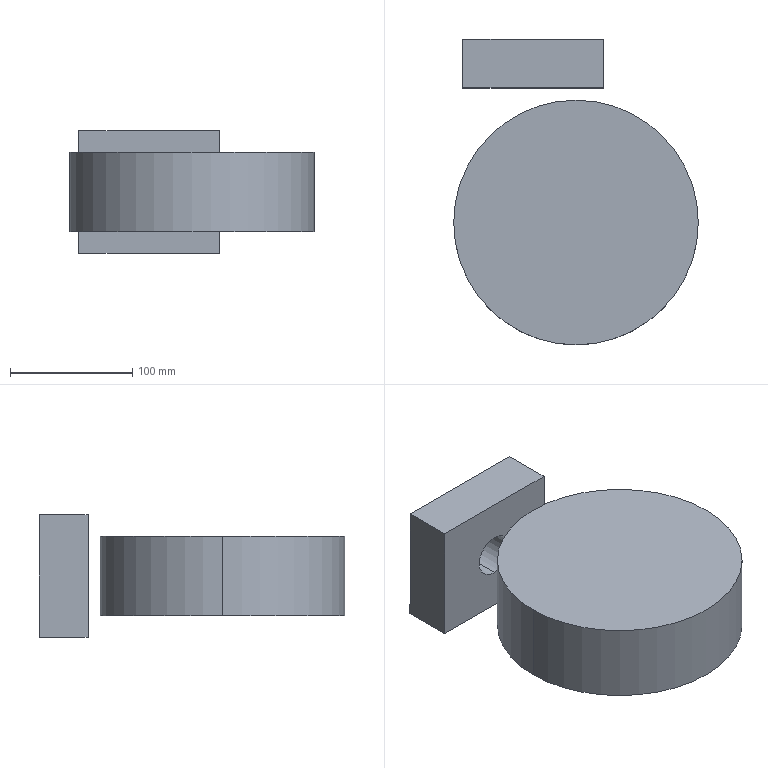Part | SolidWorks | features ICE 2, Extrusion 1 | 2 solids | 12 faces | box 200 x 250 x 100 mm | volume 2463636 mm3 | plane 8 | cylinder 4 | commonest cylinder face diameters 34.961 x2 200 x2
STEP:
#1=CARTESIAN_POINT('',(100.,0.,32.5));
#2=VERTEX_POINT('',#1);
#3=CARTESIAN_POINT('',(-100.,0.,32.5));
#4=VERTEX_POINT('',#3);
#5=CARTESIAN_POINT('',(0.,0.,32.5));
#6=DIRECTION('',(0.,0.,1.));
#7=DIRECTION('',(1.,0.,0.));
#8=AXIS2_PLACEMENT_3D('',#5,#6,#7);
#9=CIRCLE('',#8,100.);
#10=EDGE_CURVE('',#2,#4,#9,.T.);
#11=ORIENTED_EDGE('',*,*,#10,.F.);
#12=CARTESIAN_POINT('',(100.,0.,-32.5));
#13=VERTEX_POINT('',#12);
#14=CARTESIAN_POINT('',(100.,0.,32.5));
#15=DIRECTION('',(0.,0.,-1.));
#16=VECTOR('',#15,1000.);
#17=LINE('',#14,#16);
#18=EDGE_CURVE('',#2,#13,#17,.T.);
#19=ORIENTED_EDGE('',*,*,#18,.T.);
#20=CARTESIAN_POINT('',(-100.,0.,-32.5));
#21=VERTEX_POINT('',#20);
#22=CARTESIAN_POINT('',(0.,0.,-32.5));
#23=DIRECTION('',(0.,0.,1.));
#24=DIRECTION('',(1.,0.,0.));
#25=AXIS2_PLACEMENT_3D('',#22,#23,#24);
#26=CIRCLE('',#25,100.);
#27=EDGE_CURVE('',#13,#21,#26,.T.);
#28=ORIENTED_EDGE('',*,*,#27,.T.);
#29=CARTESIAN_POINT('',(-100.,0.,32.5));
#30=DIRECTION('',(0.,0.,-1.));
#31=VECTOR('',#30,1000.);
#32=LINE('',#29,#31);
#33=EDGE_CURVE('',#4,#21,#32,.T.);
#34=ORIENTED_EDGE('',*,*,#33,.F.);
#35=EDGE_LOOP('',(#11,#19,#28,#34));
#36=FACE_OUTER_BOUND('',#35,.T.);
#37=CARTESIAN_POINT('',(0.,0.,32.5));
#38=DIRECTION('',(0.,0.,-1.));
#39=DIRECTION('',(-1.,0.,0.));
#40=AXIS2_PLACEMENT_3D('',#37,#38,#39);
#41=CYLINDRICAL_SURFACE('',#40,100.);
#42=ADVANCED_FACE('',(#36),#41,.T.);
#43=ORIENTED_EDGE('',*,*,#18,.F.);
#44=CARTESIAN_POINT('',(0.,0.,32.5));
#45=DIRECTION('',(0.,0.,1.));
#46=DIRECTION('',(1.,0.,0.));
#47=AXIS2_PLACEMENT_3D('',#44,#45,#46);
#48=CIRCLE('',#47,100.);
#49=EDGE_CURVE('',#4,#2,#48,.T.);
#50=ORIENTED_EDGE('',*,*,#49,.F.);
#51=ORIENTED_EDGE('',*,*,#33,.T.);
#52=CARTESIAN_POINT('',(0.,0.,-32.5));
#53=DIRECTION('',(0.,0.,1.));
#54=DIRECTION('',(1.,0.,0.));
#55=AXIS2_PLACEMENT_3D('',#52,#53,#54);
#56=CIRCLE('',#55,100.);
#57=EDGE_CURVE('',#21,#13,#56,.T.);
#58=ORIENTED_EDGE('',*,*,#57,.T.);
#59=EDGE_LOOP('',(#43,#50,#51,#58));
#60=FACE_OUTER_BOUND('',#59,.T.);
#61=CARTESIAN_POINT('',(0.,0.,32.5));
#62=DIRECTION('',(0.,0.,-1.));
#63=DIRECTION('',(-1.,0.,0.));
#64=AXIS2_PLACEMENT_3D('',#61,#62,#63);
#65=CYLINDRICAL_SURFACE('',#64,100.);
#66=ADVANCED_FACE('',(#60),#65,.T.);
#67=ORIENTED_EDGE('',*,*,#49,.T.);
#68=ORIENTED_EDGE('',*,*,#10,.T.);
#69=EDGE_LOOP('',(#67,#68));
#70=FACE_OUTER_BOUND('',#69,.T.);
#71=CARTESIAN_POINT('',(0.,0.,32.5));
#72=DIRECTION('',(0.,0.,1.));
#73=DIRECTION('',(1.,0.,0.));
#74=AXIS2_PLACEMENT_3D('',#71,#72,#73);
#75=PLANE('',#74);
#76=ADVANCED_FACE('',(#70),#75,.T.);
#77=ORIENTED_EDGE('',*,*,#57,.F.);
#78=ORIENTED_EDGE('',*,*,#27,.F.);
#79=EDGE_LOOP('',(#77,#78));
#80=FACE_OUTER_BOUND('',#79,.T.);
#81=CARTESIAN_POINT('',(0.,0.,-32.5));
#82=DIRECTION('',(0.,0.,1.));
#83=DIRECTION('',(1.,0.,0.));
#84=AXIS2_PLACEMENT_3D('',#81,#82,#83);
#85=PLANE('',#84);
#86=ADVANCED_FACE('',(#80),#85,.F.);
#87=CLOSED_SHELL('',(#42,#66,#76,#86));
#88=MANIFOLD_SOLID_BREP('',#87);
#89=CARTESIAN_POINT('',(-35.,110.,17.481));
#90=VERTEX_POINT('',#89);
#91=CARTESIAN_POINT('',(-35.,110.,-17.481));
#92=VERTEX_POINT('',#91);
#93=CARTESIAN_POINT('',(-35.,110.,0.));
#94=DIRECTION('',(0.,-1.,0.));
#95=DIRECTION('',(-1.,0.,0.));
#96=AXIS2_PLACEMENT_3D('',#93,#94,#95);
#97=CIRCLE('',#96,17.481);
#98=EDGE_CURVE('',#90,#92,#97,.T.);
#99=ORIENTED_EDGE('',*,*,#98,.T.);
#100=CARTESIAN_POINT('',(-35.,150.,-17.481));
#101=VERTEX_POINT('',#100);
#102=CARTESIAN_POINT('',(-35.,-100.001,-17.481));
#103=DIRECTION('',(0.,1.,0.));
#104=VECTOR('',#103,1000.);
#105=LINE('',#102,#104);
#106=EDGE_CURVE('',#92,#101,#105,.T.);
#107=ORIENTED_EDGE('',*,*,#106,.T.);
#108=CARTESIAN_POINT('',(-35.,150.,17.481));
#109=VERTEX_POINT('',#108);
#110=CARTESIAN_POINT('',(-35.,150.,0.));
#111=DIRECTION('',(0.,1.,0.));
#112=DIRECTION('',(0.,0.,1.));
#113=AXIS2_PLACEMENT_3D('',#110,#111,#112);
#114=CIRCLE('',#113,17.481);
#115=EDGE_CURVE('',#101,#109,#114,.T.);
#116=ORIENTED_EDGE('',*,*,#115,.T.);
#117=CARTESIAN_POINT('',(-35.,-100.001,17.481));
#118=DIRECTION('',(0.,1.,0.));
#119=VECTOR('',#118,1000.);
#120=LINE('',#117,#119);
#121=EDGE_CURVE('',#90,#109,#120,.T.);
#122=ORIENTED_EDGE('',*,*,#121,.F.);
#123=EDGE_LOOP('',(#99,#107,#116,#122));
#124=FACE_OUTER_BOUND('',#123,.T.);
#125=CARTESIAN_POINT('',(-35.,-100.001,0.));
#126=DIRECTION('',(0.,1.,0.));
#127=DIRECTION('',(0.,0.,1.));
#128=AXIS2_PLACEMENT_3D('',#125,#126,#127);
#129=CYLINDRICAL_SURFACE('',#128,17.481);
#130=ADVANCED_FACE('',(#124),#129,.F.);
#131=CARTESIAN_POINT('',(-92.5,150.,-50.));
#132=VERTEX_POINT('',#131);
#133=CARTESIAN_POINT('',(-92.5,110.,-50.));
#134=VERTEX_POINT('',#133);
#135=CARTESIAN_POINT('',(-92.5,150.,-50.));
#136=DIRECTION('',(0.,-1.,0.));
#137=VECTOR('',#136,1000.);
#138=LINE('',#135,#137);
#139=EDGE_CURVE('',#132,#134,#138,.T.);
#140=ORIENTED_EDGE('',*,*,#139,.T.);
#141=CARTESIAN_POINT('',(-92.5,110.,50.));
#142=VERTEX_POINT('',#141);
#143=CARTESIAN_POINT('',(-92.5,110.,50.));
#144=DIRECTION('',(0.,0.,-1.));
#145=VECTOR('',#144,1000.);
#146=LINE('',#143,#145);
#147=EDGE_CURVE('',#142,#134,#146,.T.);
#148=ORIENTED_EDGE('',*,*,#147,.F.);
#149=CARTESIAN_POINT('',(-92.5,150.,50.));
#150=VERTEX_POINT('',#149);
#151=CARTESIAN_POINT('',(-92.5,150.,50.));
#152=DIRECTION('',(0.,-1.,0.));
#153=VECTOR('',#152,1000.);
#154=LINE('',#151,#153);
#155=EDGE_CURVE('',#150,#142,#154,.T.);
#156=ORIENTED_EDGE('',*,*,#155,.F.);
#157=CARTESIAN_POINT('',(-92.5,150.,50.));
#158=DIRECTION('',(0.,0.,-1.));
#159=VECTOR('',#158,1000.);
#160=LINE('',#157,#159);
#161=EDGE_CURVE('',#150,#132,#160,.T.);
#162=ORIENTED_EDGE('',*,*,#161,.T.);
#163=EDGE_LOOP('',(#140,#148,#156,#162));
#164=FACE_OUTER_BOUND('',#163,.T.);
#165=CARTESIAN_POINT('',(-92.5,150.,50.));
#166=DIRECTION('',(1.,0.,0.));
#167=DIRECTION('',(0.,1.,0.));
#168=AXIS2_PLACEMENT_3D('',#165,#166,#167);
#169=PLANE('',#168);
#170=ADVANCED_FACE('',(#164),#169,.F.);
#171=ORIENTED_EDGE('',*,*,#98,.F.);
#172=CARTESIAN_POINT('',(-35.,110.,0.));
#173=DIRECTION('',(0.,-1.,0.));
#174=DIRECTION('',(-1.,0.,0.));
#175=AXIS2_PLACEMENT_3D('',#172,#173,#174);
#176=CIRCLE('',#175,17.481);
#177=EDGE_CURVE('',#92,#90,#176,.T.);
#178=ORIENTED_EDGE('',*,*,#177,.F.);
#179=EDGE_LOOP('',(#171,#178));
#180=FACE_BOUND('',#179,.T.);
#181=CARTESIAN_POINT('',(22.5,110.,-50.));
#182=VERTEX_POINT('',#181);
#183=CARTESIAN_POINT('',(-92.5,110.,-50.));
#184=DIRECTION('',(1.,0.,0.));
#185=VECTOR('',#184,1000.);
#186=LINE('',#183,#185);
#187=EDGE_CURVE('',#134,#182,#186,.T.);
#188=ORIENTED_EDGE('',*,*,#187,.T.);
#189=CARTESIAN_POINT('',(22.5,110.,50.));
#190=VERTEX_POINT('',#189);
#191=CARTESIAN_POINT('',(22.5,110.,50.));
#192=DIRECTION('',(0.,0.,-1.));
#193=VECTOR('',#192,1000.);
#194=LINE('',#191,#193);
#195=EDGE_CURVE('',#190,#182,#194,.T.);
#196=ORIENTED_EDGE('',*,*,#195,.F.);
#197=CARTESIAN_POINT('',(-92.5,110.,50.));
#198=DIRECTION('',(1.,0.,0.));
#199=VECTOR('',#198,1000.);
#200=LINE('',#197,#199);
#201=EDGE_CURVE('',#142,#190,#200,.T.);
#202=ORIENTED_EDGE('',*,*,#201,.F.);
#203=ORIENTED_EDGE('',*,*,#147,.T.);
#204=EDGE_LOOP('',(#188,#196,#202,#203));
#205=FACE_OUTER_BOUND('',#204,.T.);
#206=CARTESIAN_POINT('',(-92.5,110.,50.));
#207=DIRECTION('',(0.,1.,0.));
#208=DIRECTION('',(-1.,0.,0.));
#209=AXIS2_PLACEMENT_3D('',#206,#207,#208);
#210=PLANE('',#209);
#211=ADVANCED_FACE('',(#180,#205),#210,.F.);
#212=CARTESIAN_POINT('',(22.5,150.,-50.));
#213=VERTEX_POINT('',#212);
#214=CARTESIAN_POINT('',(22.5,150.,-50.));
#215=DIRECTION('',(0.,1.,0.));
#216=VECTOR('',#215,1000.);
#217=LINE('',#214,#216);
#218=EDGE_CURVE('',#182,#213,#217,.T.);
#219=ORIENTED_EDGE('',*,*,#218,.T.);
#220=CARTESIAN_POINT('',(22.5,150.,50.));
#221=VERTEX_POINT('',#220);
#222=CARTESIAN_POINT('',(22.5,150.,50.));
#223=DIRECTION('',(0.,0.,-1.));
#224=VECTOR('',#223,1000.);
#225=LINE('',#222,#224);
#226=EDGE_CURVE('',#221,#213,#225,.T.);
#227=ORIENTED_EDGE('',*,*,#226,.F.);
#228=CARTESIAN_POINT('',(22.5,150.,50.));
#229=DIRECTION('',(0.,1.,0.));
#230=VECTOR('',#229,1000.);
#231=LINE('',#228,#230);
#232=EDGE_CURVE('',#190,#221,#231,.T.);
#233=ORIENTED_EDGE('',*,*,#232,.F.);
#234=ORIENTED_EDGE('',*,*,#195,.T.);
#235=EDGE_LOOP('',(#219,#227,#233,#234));
#236=FACE_OUTER_BOUND('',#235,.T.);
#237=CARTESIAN_POINT('',(22.5,150.,50.));
#238=DIRECTION('',(-1.,0.,0.));
#239=DIRECTION('',(0.,0.,1.));
#240=AXIS2_PLACEMENT_3D('',#237,#238,#239);
#241=PLANE('',#240);
#242=ADVANCED_FACE('',(#236),#241,.F.);
#243=CARTESIAN_POINT('',(-35.,150.,0.));
#244=DIRECTION('',(0.,1.,0.));
#245=DIRECTION('',(0.,0.,1.));
#246=AXIS2_PLACEMENT_3D('',#243,#244,#245);
#247=CIRCLE('',#246,17.481);
#248=EDGE_CURVE('',#109,#101,#247,.T.);
#249=ORIENTED_EDGE('',*,*,#248,.F.);
#250=ORIENTED_EDGE('',*,*,#115,.F.);
#251=EDGE_LOOP('',(#249,#250));
#252=FACE_BOUND('',#251,.T.);
#253=CARTESIAN_POINT('',(-92.5,150.,-50.));
#254=DIRECTION('',(-1.,0.,0.));
#255=VECTOR('',#254,1000.);
#256=LINE('',#253,#255);
#257=EDGE_CURVE('',#213,#132,#256,.T.);
#258=ORIENTED_EDGE('',*,*,#257,.T.);
#259=ORIENTED_EDGE('',*,*,#161,.F.);
#260=CARTESIAN_POINT('',(-92.5,150.,50.));
#261=DIRECTION('',(-1.,0.,0.));
#262=VECTOR('',#261,1000.);
#263=LINE('',#260,#262);
#264=EDGE_CURVE('',#221,#150,#263,.T.);
#265=ORIENTED_EDGE('',*,*,#264,.F.);
#266=ORIENTED_EDGE('',*,*,#226,.T.);
#267=EDGE_LOOP('',(#258,#259,#265,#266));
#268=FACE_OUTER_BOUND('',#267,.T.);
#269=CARTESIAN_POINT('',(-92.5,150.,50.));
#270=DIRECTION('',(0.,-1.,0.));
#271=DIRECTION('',(1.,0.,0.));
#272=AXIS2_PLACEMENT_3D('',#269,#270,#271);
#273=PLANE('',#272);
#274=ADVANCED_FACE('',(#252,#268),#273,.F.);
#275=ORIENTED_EDGE('',*,*,#155,.T.);
#276=ORIENTED_EDGE('',*,*,#201,.T.);
#277=ORIENTED_EDGE('',*,*,#232,.T.);
#278=ORIENTED_EDGE('',*,*,#264,.T.);
#279=EDGE_LOOP('',(#275,#276,#277,#278));
#280=FACE_OUTER_BOUND('',#279,.T.);
#281=CARTESIAN_POINT('',(0.,0.,50.));
#282=DIRECTION('',(0.,0.,1.));
#283=DIRECTION('',(1.,0.,0.));
#284=AXIS2_PLACEMENT_3D('',#281,#282,#283);
#285=PLANE('',#284);
#286=ADVANCED_FACE('',(#280),#285,.T.);
#287=ORIENTED_EDGE('',*,*,#139,.F.);
#288=ORIENTED_EDGE('',*,*,#257,.F.);
#289=ORIENTED_EDGE('',*,*,#218,.F.);
#290=ORIENTED_EDGE('',*,*,#187,.F.);
#291=EDGE_LOOP('',(#287,#288,#289,#290));
#292=FACE_OUTER_BOUND('',#291,.T.);
#293=CARTESIAN_POINT('',(0.,0.,-50.));
#294=DIRECTION('',(0.,0.,1.));
#295=DIRECTION('',(1.,0.,0.));
#296=AXIS2_PLACEMENT_3D('',#293,#294,#295);
#297=PLANE('',#296);
#298=ADVANCED_FACE('',(#292),#297,.F.);
#299=ORIENTED_EDGE('',*,*,#106,.F.);
#300=ORIENTED_EDGE('',*,*,#177,.T.);
#301=ORIENTED_EDGE('',*,*,#121,.T.);
#302=ORIENTED_EDGE('',*,*,#248,.T.);
#303=EDGE_LOOP('',(#299,#300,#301,#302));
#304=FACE_OUTER_BOUND('',#303,.T.);
#305=CARTESIAN_POINT('',(-35.,-100.001,0.));
#306=DIRECTION('',(0.,1.,0.));
#307=DIRECTION('',(0.,0.,1.));
#308=AXIS2_PLACEMENT_3D('',#305,#306,#307);
#309=CYLINDRICAL_SURFACE('',#308,17.481);
#310=ADVANCED_FACE('',(#304),#309,.F.);
#311=CLOSED_SHELL('',(#130,#170,#211,#242,#274,#286,#298,#310));
#312=MANIFOLD_SOLID_BREP('',#311);
#313=CARTESIAN_POINT('',(0.,0.,0.));
#314=DIRECTION('',(0.,0.,1.));
#315=DIRECTION('',(1.,0.,0.));
#316=AXIS2_PLACEMENT_3D('',#313,#314,#315);
#317=(LENGTH_UNIT()NAMED_UNIT(*)SI_UNIT(.MILLI.,.METRE.));
#318=UNCERTAINTY_MEASURE_WITH_UNIT(LENGTH_MEASURE(0.00001),#317,'','');
#319=(NAMED_UNIT(*)PLANE_ANGLE_UNIT()SI_UNIT($,.RADIAN.));
#320=(NAMED_UNIT(*)SI_UNIT($,.STERADIAN.)SOLID_ANGLE_UNIT());
#321=(GEOMETRIC_REPRESENTATION_CONTEXT(3)GLOBAL_UNCERTAINTY_ASSIGNED_CONTEXT((#318))GLOBAL_UNIT_ASSIGNED_CONTEXT((#317,#319,#320))REPRESENTATION_CONTEXT('',''));
#322=ADVANCED_BREP_SHAPE_REPRESENTATION('',(#88,#312,#316),#321);